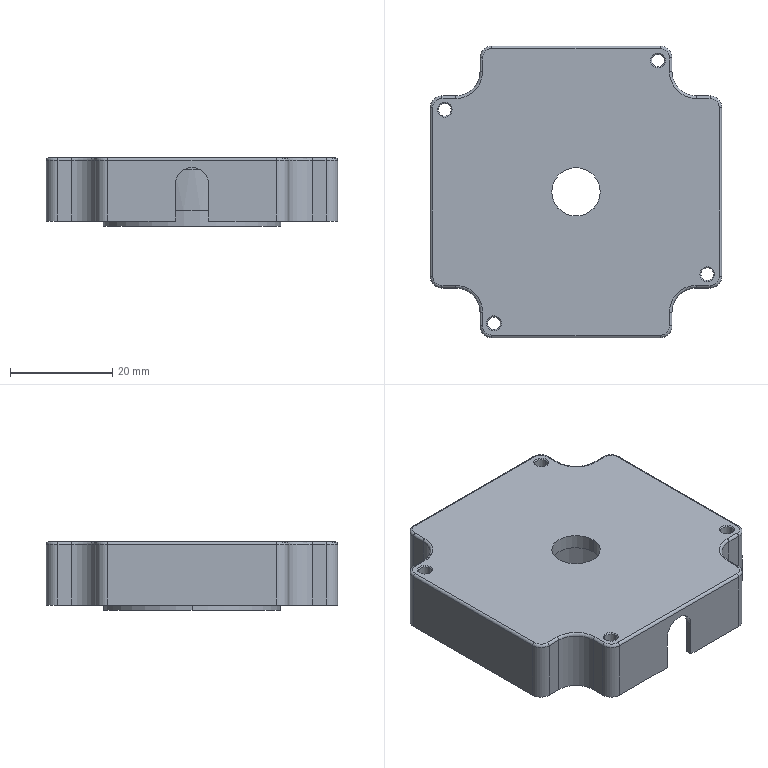Part | NX | features BREP 1 | 1 solid | 92 faces | box 57.15 x 57.15 x 13.4 mm | volume 17419 mm3 | cylinder 46 | plane 26 | torus 12 | cone 8 | commonest cylinder face diameters 1 x12 2.5 x8 4.6 x8 9.5 x6 53.8 x3 22 x2